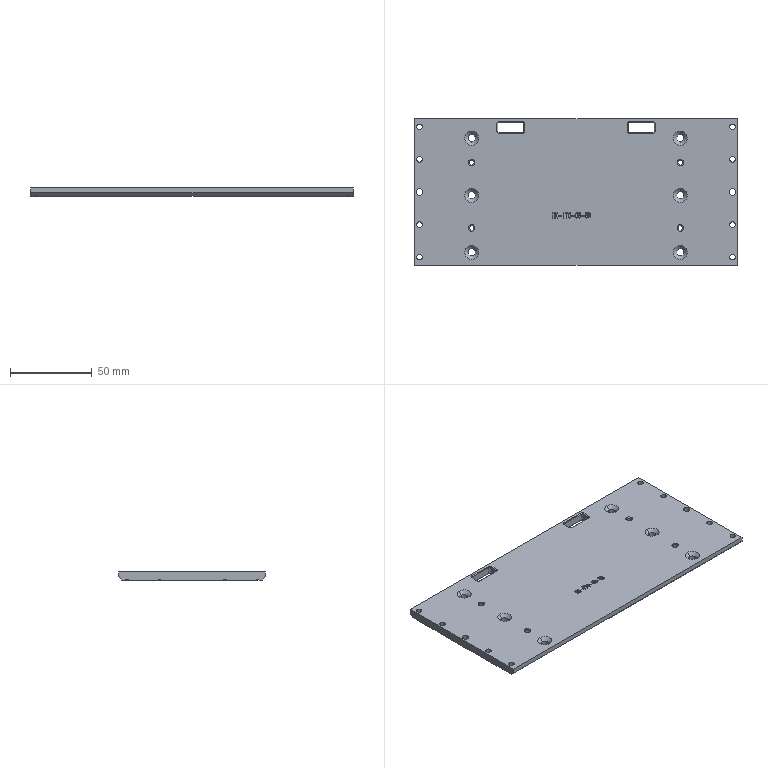NC program | NX | posted with a generic post | part box 198 x 90 x 5 mm
Lines 1 to 838 of 3871:
N10 G17 G21 G94 G90
(ZLEVEL_PROFILE_COPY_1_COPY_COPY_COPY_1_COPY , TOOL : D6A45)
N12 T01 M6
N14 G54
N16 G17 G0 G90 X65.223 Y29.3 S9500 M3
N18 G43 Z30. H1
N20 Z1.5
N22 G94 G1 X65.232 Y29.302 F1000.
N24 X65.925 Y29.611 Z1.46
N26 X66.546 Y30.049 Z1.42
N28 X67.07 Y30.598 Z1.38
N30 X67.477 Y31.239 Z1.34
N32 X67.753 Y31.946 Z1.301
N34 X67.886 Y32.694 Z1.261
N36 X67.871 Y33.453 Z1.221
N38 X67.71 Y34.195 Z1.181
N40 X67.501 Y34.712 Z1.152
N42 X67.152 Y35.293 Z1.116
N44 X66.707 Y35.804 Z1.081
N46 X66.181 Y36.23 Z1.045
N48 X65.589 Y36.559 Z1.01
N50 X64.948 Y36.78 Z0.974
N52 X64.279 Y36.887 Z0.939
N54 X63.721 Z0.91
N56 X62.989 Y36.764 Z0.871
N58 X62.293 Y36.503 Z0.832
N60 X61.659 Y36.116 Z0.793
N62 X61.111 Y35.615 Z0.754
N64 X60.767 Y35.176 Z0.725
N66 X60.406 Y34.508 Z0.685
N68 X60.182 Y33.782 Z0.645
N70 X60.103 Y33.027 Z0.605
N72 X60.172 Y32.271 Z0.566
N74 X60.386 Y31.543 Z0.526
N76 X60.737 Y30.869 Z0.486
N78 X61.212 Y30.277 Z0.446
N80 X61.792 Y29.788 Z0.406
N82 X62.457 Y29.421 Z0.367
N84 X63.18 Y29.19 Z0.327
N86 X63.733 Y29.112 Z0.298
N88 X64.492 Y29.134 Z0.258
N90 X65.232 Y29.302 Z0.218
N92 X65.925 Y29.611 Z0.178
N94 X66.546 Y30.049 Z0.138
N96 X67.07 Y30.598 Z0.099
N98 X67.477 Y31.239 Z0.059
N100 X67.753 Y31.946 Z0.019
N102 X67.886 Y32.694 Z-0.021
N104 X67.871 Y33.453 Z-0.06
N106 X67.71 Y34.195 Z-0.1
N108 X67.501 Y34.712 Z-0.129
N110 X67.152 Y35.293 Z-0.165
N112 X66.707 Y35.804 Z-0.201
N114 X66.181 Y36.23 Z-0.236
N116 X65.589 Y36.559 Z-0.272
N118 X64.948 Y36.78 Z-0.307
N120 X64.279 Y36.887 Z-0.343
N122 X64. Z-0.357
N124 G3 X60.113 Y33. R3.887 F1300.
N126 X64. Y36.887 R-3.887
N128 G1 X63.499 Y36.847 Z-0.365
N130 X63.008 Y36.742 Z-0.373
N132 X62.536 Y36.576 Z-0.38
N134 X62.09 Y36.35 Z-0.388
N136 X61.678 Y36.069 Z-0.396
N138 X61.307 Y35.738 Z-0.403
N140 X60.982 Y35.362 Z-0.411
N142 X60.689 Y34.915 Z-0.419
N144 X60.463 Y34.432 Z-0.427
N146 X60.362 Y34.127 Z-0.432
N148 X60.306 Y33.924 Z-0.435
N150 X60.263 Y33.662 Z-0.439
N152 X60.222 Y33.4 Z-0.444
N154 X60.215 Y33.135 Z-0.448
N156 X60.213 Y32.87 Z-0.452
N158 X60.24 Y32.608 Z-0.456
N160 X60.276 Y32.346 Z-0.46
N162 X60.337 Y32.09 Z-0.464
N164 X60.412 Y31.837 Z-0.468
N166 X60.506 Y31.591 Z-0.472
N168 X60.616 Y31.352 Z-0.476
N170 X60.741 Y31.122 Z-0.48
N172 X60.885 Y30.902 Z-0.484
N174 X61.042 Y30.692 Z-0.488
N176 X61.213 Y30.494 Z-0.492
N178 X61.398 Y30.31 Z-0.496
N180 X61.594 Y30.136 Z-0.5
N182 X61.804 Y29.982 Z-0.504
N184 X62.019 Y29.835 Z-0.508
N186 X62.249 Y29.713 Z-0.512
N188 X62.482 Y29.597 Z-0.516
N190 X62.727 Y29.51 Z-0.52
N192 X62.973 Y29.426 Z-0.524
N194 X63.227 Y29.375 Z-0.528
N196 X63.481 Y29.326 Z-0.532
N198 X63.739 Y29.311 Z-0.536
N200 X63.998 Y29.297 Z-0.54
N202 X64.255 Y29.319 Z-0.544
N204 X64.512 Y29.341 Z-0.548
N206 X64.817 Y29.403 Z-0.553
N208 X65.014 Y29.456 Z-0.556
N210 X65.254 Y29.546 Z-0.56
N212 X65.494 Y29.639 Z-0.564
N214 X65.719 Y29.76 Z-0.568
N216 X65.943 Y29.886 Z-0.572
N218 X66.15 Y30.036 Z-0.576
N220 X66.351 Y30.194 Z-0.579
N222 X66.537 Y30.369 Z-0.583
N224 X66.713 Y30.554 Z-0.587
N226 X66.873 Y30.752 Z-0.591
N228 X67.02 Y30.96 Z-0.595
N230 X67.153 Y31.176 Z-0.599
N232 X67.267 Y31.403 Z-0.603
N234 X67.367 Y31.636 Z-0.607
N236 X67.451 Y31.876 Z-0.611
N238 X67.515 Y32.12 Z-0.615
N240 X67.566 Y32.368 Z-0.619
N242 X67.594 Y32.619 Z-0.622
N244 X67.612 Y32.871 Z-0.626
N246 X67.603 Y33.123 Z-0.63
N248 X67.588 Y33.374 Z-0.634
N250 X67.542 Y33.621 Z-0.638
N252 X67.493 Y33.868 Z-0.642
N254 X67.413 Y34.106 Z-0.646
N256 X67.331 Y34.343 Z-0.649
N258 X67.119 Y34.766 Z-0.657
N260 X66.854 Y35.156 Z-0.664
N262 X66.621 Y35.426 Z-0.669
N264 X66.541 Y35.508 Z-0.671
N266 X66.363 Y35.662 Z-0.675
N268 X66.184 Y35.815 Z-0.678
N270 X65.988 Y35.944 Z-0.682
N272 X65.791 Y36.072 Z-0.686
N274 X65.58 Y36.173 Z-0.689
N276 X65.369 Y36.275 Z-0.693
N278 X64.924 Y36.419 Z-0.7
N280 X64.465 Y36.505 Z-0.707
N282 X64.233 Y36.516 Z-0.711
N284 X64. Y36.526 Z-0.714
N286 X63.753 Y36.507 Z-0.719
N288 X63.505 Y36.483 Z-0.723
N290 X63.263 Y36.429 Z-0.727
N292 X63.023 Y36.37 Z-0.731
N294 X62.791 Y36.284 Z-0.735
N296 X62.562 Y36.191 Z-0.74
N298 X62.344 Y36.075 Z-0.744
N300 X62.131 Y35.95 Z-0.748
N302 X61.932 Y35.806 Z-0.752
N304 X61.74 Y35.651 Z-0.756
N306 X61.562 Y35.482 Z-0.76
N308 X61.397 Y35.301 Z-0.765
N310 X61.243 Y35.11 Z-0.769
N312 X61.106 Y34.907 Z-0.773
N314 X60.983 Y34.696 Z-0.777
N316 X60.873 Y34.478 Z-0.781
N318 X60.784 Y34.251 Z-0.785
N320 X60.704 Y34.021 Z-0.79
N322 X60.646 Y33.77 Z-0.794
N324 X60.597 Y33.517 Z-0.798
N326 X60.579 Y33.26 Z-0.803
N328 X60.566 Y33.004 Z-0.807
N330 X60.587 Y32.748 Z-0.811
N332 X60.614 Y32.493 Z-0.816
N334 X60.67 Y32.244 Z-0.82
N336 X60.735 Y31.997 Z-0.825
N338 X60.826 Y31.759 Z-0.829
N340 X60.929 Y31.525 Z-0.833
N342 X61.051 Y31.302 Z-0.838
N344 X61.19 Y31.089 Z-0.842
N346 X61.346 Y30.889 Z-0.846
N348 X61.513 Y30.697 Z-0.85
N350 X61.698 Y30.525 Z-0.855
N352 X61.889 Y30.359 Z-0.859
N354 X62.098 Y30.217 Z-0.863
N356 X62.31 Y30.08 Z-0.868
N358 X62.538 Y29.973 Z-0.872
N360 X62.768 Y29.87 Z-0.876
N362 X62.898 Y29.825 Z-0.879
N364 X63.073 Y29.774 Z-0.882
N366 X63.25 Y29.73 Z-0.885
N368 X63.497 Y29.69 Z-0.889
N370 X63.746 Y29.663 Z-0.893
N372 X63.996 Y29.657 Z-0.898
N374 X64.246 Y29.671 Z-0.902
N376 X64.493 Y29.705 Z-0.906
N378 X64.737 Y29.753 Z-0.91
N380 X64.975 Y29.826 Z-0.915
N382 X65.21 Y29.907 Z-0.919
N384 X65.433 Y30.015 Z-0.923
N386 X65.654 Y30.128 Z-0.927
N388 X65.857 Y30.269 Z-0.931
N390 X66.057 Y30.415 Z-0.936
N392 X66.238 Y30.582 Z-0.94
N394 X66.413 Y30.756 Z-0.944
N396 X66.569 Y30.946 Z-0.948
N398 X66.714 Y31.145 Z-0.952
N400 X66.842 Y31.355 Z-0.957
N402 X66.952 Y31.574 Z-0.961
N404 X67.045 Y31.801 Z-0.965
N406 X67.124 Y32.033 Z-0.969
N408 X67.179 Y32.27 Z-0.973
N410 X67.225 Y32.51 Z-0.977
N412 X67.243 Y32.753 Z-0.982
N414 X67.255 Y32.996 Z-0.986
N416 X67.235 Y33.238 Z-0.99
N418 X67.21 Y33.48 Z-0.994
N420 X67.185 Y33.612 Z-0.996
N422 X67.142 Y33.782 Z-0.999
N424 X67.094 Y33.951 Z-1.002
N426 X67.008 Y34.176 Z-1.006
N428 X66.911 Y34.398 Z-1.01
N430 X66.795 Y34.609 Z-1.014
N432 X66.663 Y34.811 Z-1.019
N434 X66.516 Y35.002 Z-1.023
N436 X66.357 Y35.182 Z-1.027
N438 X66.198 Y35.334 Z-1.031
N440 X66.032 Y35.479 Z-1.034
N442 X65.853 Y35.606 Z-1.038
N444 X65.669 Y35.727 Z-1.042
N446 X65.475 Y35.828 Z-1.045
N448 X65.277 Y35.923 Z-1.049
N450 X65.071 Y35.996 Z-1.053
N452 X64.863 Y36.064 Z-1.057
N454 X64.65 Y36.107 Z-1.06
N456 X64.435 Y36.147 Z-1.064
N458 X64.218 Y36.159 Z-1.068
N460 X64. Y36.168 Z-1.071
N462 X63.775 Y36.15 Z-1.076
N464 X63.551 Y36.129 Z-1.08
N466 X63.331 Y36.079 Z-1.084
N468 X63.113 Y36.023 Z-1.089
N470 X62.903 Y35.945 Z-1.093
N472 X62.696 Y35.859 Z-1.097
N474 X62.499 Y35.753 Z-1.101
N476 X62.307 Y35.637 Z-1.106
N478 X62.127 Y35.506 Z-1.11
N480 X61.955 Y35.363 Z-1.114
N482 X61.788 Y35.201 Z-1.119
N484 X61.632 Y35.027 Z-1.123
N486 X61.494 Y34.84 Z-1.127
N488 X61.364 Y34.646 Z-1.132
N490 X61.334 Y34.595 Z-1.133
N492 X61.245 Y34.413 Z-1.137
N494 X61.156 Y34.232 Z-1.141
N496 X61.082 Y34.012 Z-1.145
N498 X61.011 Y33.792 Z-1.149
N500 X60.972 Y33.565 Z-1.154
N502 X60.937 Y33.337 Z-1.158
N504 X60.929 Y33.107 Z-1.163
N506 Y32.877 Z-1.167
N508 X60.954 Y32.649 Z-1.171
N510 X60.991 Y32.422 Z-1.176
N512 X61.046 Y32.2 Z-1.18
N514 X61.118 Y31.983 Z-1.184
N516 X61.209 Y31.774 Z-1.189
N518 X61.31 Y31.569 Z-1.193
N520 X61.432 Y31.377 Z-1.198
N522 X61.56 Y31.189 Z-1.202
N524 X61.71 Y31.019 Z-1.206
N526 X61.862 Y30.851 Z-1.21
N528 X62.036 Y30.706 Z-1.215
N530 X62.212 Y30.564 Z-1.219
N532 X62.404 Y30.445 Z-1.223
N534 X62.599 Y30.333 Z-1.228
N536 X62.805 Y30.242 Z-1.232
N538 X63.015 Y30.162 Z-1.236
N540 X63.231 Y30.1 Z-1.241
N542 X63.451 Y30.055 Z-1.245
N544 X63.673 Y30.029 Z-1.249
N546 X63.896 Y30.014 Z-1.253
N548 X63.953 Z-1.254
N550 X64.147 Y30.027 Z-1.258
N552 X64.341 Y30.041 Z-1.262
N554 X64.559 Y30.084 Z-1.266
N556 X64.777 Y30.131 Z-1.27
N558 X64.985 Y30.208 Z-1.275
N560 X65.192 Y30.288 Z-1.279
N562 X65.387 Y30.393 Z-1.283
N564 X65.578 Y30.503 Z-1.287
N566 X65.756 Y30.633 Z-1.291
N568 X65.927 Y30.773 Z-1.296
N570 X66.085 Y30.926 Z-1.3
N572 X66.231 Y31.09 Z-1.304
N574 X66.361 Y31.267 Z-1.308
N576 X66.484 Y31.448 Z-1.312
N578 X66.584 Y31.643 Z-1.316
N580 X66.68 Y31.839 Z-1.321
N582 X66.749 Y32.046 Z-1.325
N584 X66.816 Y32.254 Z-1.329
N586 X66.852 Y32.468 Z-1.333
N588 X66.887 Y32.683 Z-1.337
N590 X66.893 Y32.899 Z-1.341
N592 Y33.116 Z-1.345
N594 X66.869 Y33.331 Z-1.35
N596 X66.836 Y33.545 Z-1.354
N598 X66.78 Y33.758 Z-1.358
N600 X66.711 Y33.969 Z-1.362
N602 X66.621 Y34.17 Z-1.366
N604 X66.524 Y34.368 Z-1.371
N606 X66.508 Y34.397
N608 X66.393 Y34.565 Z-1.375
N610 X66.279 Y34.733 Z-1.379
N612 X66.132 Y34.895 Z-1.383
N614 X65.981 Y35.055 Z-1.387
N616 X65.813 Y35.193 Z-1.391
N618 X65.639 Y35.327 Z-1.396
N620 X65.453 Y35.439 Z-1.4
N622 X65.261 Y35.542 Z-1.404
N624 X65.06 Y35.626 Z-1.408
N626 X64.855 Y35.698 Z-1.412
N628 X64.644 Y35.746 Z-1.416
N630 X64.431 Y35.788 Z-1.42
N632 X64.216 Y35.803 Z-1.424
N634 X64. Y35.814 Z-1.429
N636 X63.794 Y35.795 Z-1.433
N638 X63.588 Y35.774 Z-1.438
N640 X63.387 Y35.726 Z-1.442
N642 X63.188 Y35.675 Z-1.446
N644 X62.996 Y35.6 Z-1.451
N646 X62.807 Y35.519 Z-1.455
N648 X62.629 Y35.419 Z-1.46
N650 X62.455 Y35.309 Z-1.464
N652 X62.294 Y35.184 Z-1.469
N654 X62.139 Y35.051 Z-1.473
N656 X62.014 Y34.925 Z-1.477
N658 X61.864 Y34.75 Z-1.482
N660 X61.751 Y34.581 Z-1.486
N662 X61.638 Y34.413 Z-1.491
N664 X61.537 Y34.209 Z-1.495
N666 X61.451 Y34.012 Z-1.5
N668 X61.389 Y33.801 Z-1.505
N670 X61.331 Y33.588 Z-1.51
N672 X61.3 Y33.371 Z-1.514
N674 X61.281 Y33.152 Z-1.519
N676 X61.287 Y32.933 Z-1.524
N678 X61.301 Y32.714 Z-1.529
N680 X61.344 Y32.501 Z-1.533
N682 X61.39 Y32.288 Z-1.538
N684 X61.465 Y32.078 Z-1.543
N686 X61.547 Y31.882 Z-1.547
N688 X61.652 Y31.693 Z-1.552
N690 X61.766 Y31.509 Z-1.557
N692 X61.9 Y31.339 Z-1.561
N694 X62.041 Y31.176 Z-1.566
N696 X62.201 Y31.033 Z-1.571
N698 X62.364 Y30.892 Z-1.575
N700 X62.548 Y30.771 Z-1.58
N702 X62.728 Y30.665 Z-1.585
N704 X62.924 Y30.58 Z-1.589
N706 X63.122 Y30.501 Z-1.594
N708 X63.356 Y30.435 Z-1.599
N710 X63.536 Y30.401 Z-1.603
N712 X63.747 Y30.383 Z-1.608
N714 X63.959 Y30.369 Z-1.612
N716 X64.17 Y30.386 Z-1.617
N718 X64.38 Y30.405 Z-1.621
N720 X64.59 Y30.451 Z-1.626
N722 X64.789 Y30.509 Z-1.631
N724 X64.984 Y30.587 Z-1.635
N726 X65.174 Y30.676 Z-1.64
N728 X65.352 Y30.786 Z-1.644
N730 X65.526 Y30.901 Z-1.649
N732 X65.682 Y31.04 Z-1.653
N734 X65.837 Y31.18 Z-1.658
N736 X65.974 Y31.341 Z-1.662
N738 X66.098 Y31.503 Z-1.667
N740 X66.204 Y31.681 Z-1.671
N742 X66.302 Y31.863 Z-1.676
N744 X66.378 Y32.055 Z-1.68
N746 X66.447 Y32.25 Z-1.685
N748 X66.488 Y32.451 Z-1.689
N750 X66.527 Y32.653 Z-1.693
N752 X66.539 Y32.862 Z-1.698
N754 X66.541 Y33.063 Z-1.702
N756 X66.517 Y33.266 Z-1.707
N758 X66.488 Y33.468 Z-1.711
N760 X66.431 Y33.692 Z-1.716
N762 X66.373 Y33.858 Z-1.72
N764 X66.287 Y34.042 Z-1.724
N766 X66.198 Y34.224 Z-1.729
N768 X65.981 Y34.537 Z-1.737
N770 X65.85 Y34.675 Z-1.741
N772 X65.72 Y34.813 Z-1.745
N774 X65.572 Y34.93 Z-1.749
N776 X65.421 Y35.046 Z-1.753
N778 X65.259 Y35.141 Z-1.757
N780 X65.092 Y35.229 Z-1.761
N782 X64.917 Y35.299 Z-1.766
N784 X64.74 Y35.361 Z-1.77
N786 X64.557 Y35.401 Z-1.774
N788 X64.373 Y35.438 Z-1.778
N790 X64.187 Y35.448 Z-1.782
N792 X64. Y35.459 Z-1.786
N794 X63.805 Y35.439 Z-1.791
N796 X63.609 Y35.417 Z-1.796
N798 X63.42 Y35.369 Z-1.8
N800 X63.232 Y35.314 Z-1.805
N802 X63.052 Y35.239 Z-1.81
N804 X62.877 Y35.154 Z-1.815
N806 X62.714 Y35.048 Z-1.82
N808 X62.553 Y34.94 Z-1.825
N810 X62.411 Y34.809 Z-1.83
N812 X62.269 Y34.677 Z-1.834
N814 X62.185 Y34.578 Z-1.838
N816 X62.097 Y34.463 Z-1.841
N818 X62.014 Y34.345 Z-1.845
N820 X61.912 Y34.163 Z-1.85
N822 X61.819 Y33.976 Z-1.855
N824 X61.745 Y33.765 Z-1.861
N826 X61.693 Y33.58 Z-1.866
N828 X61.662 Y33.375 Z-1.871
N830 X61.639 Y33.169 Z-1.876
N832 X61.634 Y33.02 Z-1.88
N834 X61.638 Y32.946 Z-1.882
N836 X61.654 Y32.758 Z-1.886
N838 X61.696 Y32.557 Z-1.891
N840 X61.742 Y32.357 Z-1.897
N842 X61.789 Y32.227 Z-1.9
N844 X61.836 Y32.099 Z-1.903
N846 X61.898 Y31.979 Z-1.907
N848 X62.001 Y31.804 Z-1.912
N850 X62.115 Y31.635 Z-1.917
N852 X62.257 Y31.469 Z-1.922
N854 X62.387 Y31.336 Z-1.927
N856 X62.544 Y31.209 Z-1.932
N858 X62.707 Y31.09 Z-1.937
N860 X62.829 Y31.014 Z-1.941
N862 X62.893 Y30.981 Z-1.943
N864 X62.949 Y30.955 Z-1.944
N866 X63.062 Y30.903 Z-1.947
N868 X63.252 Y30.84 Z-1.952
N870 X63.443 Y30.781 Z-1.957
N872 X63.564 Y30.758 Z-1.96
N874 X63.7 Y30.74 Z-1.964
N876 X63.837 Y30.728 Z-1.967
N878 X64.035 Y30.731 Z-1.972
N880 X64.233 Y30.744 Z-1.977
N882 X64.443 Y30.783 Z-1.982
N884 X64.618 Y30.829 Z-1.987
N886 X64.802 Y30.899 Z-1.992
N888 X64.982 Y30.978 Z-1.997
N890 X65.104 Y31.043 Z-2.
N892 X65.163 Y31.081 Z-2.002
N894 X65.213 Y31.116 Z-2.004
N896 X65.312 Y31.187 Z-2.007
N898 X65.458 Y31.316 Z-2.011
N900 X65.6 Y31.449 Z-2.016
N902 X65.688 Y31.551 Z-2.02
N904 X65.77 Y31.651 Z-2.023
N906 X65.837 Y31.756 Z-2.026
N908 X65.931 Y31.924 Z-2.031
N910 X66.016 Y32.098 Z-2.036
N912 X66.087 Y32.294 Z-2.041
N914 X66.133 Y32.464 Z-2.045
N916 X66.163 Y32.653 Z-2.05
N918 X66.184 Y32.843 Z-2.055
N920 X66.189 Y32.979 Z-2.058
N922 X66.186 Y33.046 Z-2.06
N924 X66.18 Y33.105 Z-2.061
N926 X66.169 Y33.224 Z-2.064
N928 X66.131 Y33.41 Z-2.069
N930 X66.088 Y33.594 Z-2.074
N932 X66.05 Y33.706 Z-2.077
N934 X66.004 Y33.813 Z-2.08
N936 X65.957 Y33.919 Z-2.083
N938 X65.871 Y34.071 Z-2.087
N940 X65.776 Y34.217 Z-2.091
N942 X65.667 Y34.351 Z-2.096
N944 X65.551 Y34.481 Z-2.1
N946 X65.421 Y34.594 Z-2.104
N948 X65.287 Y34.705 Z-2.109
N950 X65.141 Y34.796 Z-2.113
N952 X64.992 Y34.882 Z-2.117
N954 X64.835 Y34.95 Z-2.122
N956 X64.673 Y35.009 Z-2.126
N958 X64.508 Y35.05 Z-2.13
N960 X64.34 Y35.083 Z-2.134
N962 X64.17 Y35.095 Z-2.139
N964 X64. Y35.102 Z-2.143
N966 X63.822 Y35.085 Z-2.148
N968 X63.644 Y35.061 Z-2.153
N970 X63.521 Y35.034 Z-2.157
N972 X63.459 Y35.019 Z-2.159
N974 X63.407 Y35. Z-2.161
N976 X63.302 Y34.96 Z-2.164
N978 X63.141 Y34.886 Z-2.169
N980 X62.983 Y34.804 Z-2.174
N982 X62.826 Y34.7 Z-2.18
N984 X62.698 Y34.597 Z-2.185
N986 X62.572 Y34.474 Z-2.19
N988 X62.453 Y34.345 Z-2.195
N990 X62.345 Y34.2 Z-2.201
N992 X62.236 Y34.022 Z-2.207
N994 X62.172 Y33.891 Z-2.211
N996 X62.119 Y33.773 Z-2.215
N998 X62.085 Y33.666 Z-2.218
N1000 X62.039 Y33.479 Z-2.224
N1002 X62.005 Y33.29 Z-2.23
N1004 X61.994 Y33.152 Z-2.234
N1006 X61.989 Y33.025 Z-2.238
N1008 X61.997 Y32.908 Z-2.241
N1010 X62.023 Y32.719 Z-2.247
N1012 X62.062 Y32.533 Z-2.252
N1014 X62.103 Y32.4 Z-2.256
N1016 X62.147 Y32.282 Z-2.26
N1018 X62.195 Y32.179 Z-2.264
N1020 X62.287 Y32.015 Z-2.269
N1022 X62.392 Y31.859 Z-2.275
N1024 X62.48 Y31.75 Z-2.279
N1026 X62.565 Y31.659 Z-2.282
N1028 X62.645 Y31.583 Z-2.286
N1030 X62.79 Y31.467 Z-2.291
N1032 X62.943 Y31.361 Z-2.297
N1034 X63.061 Y31.294 Z-2.301
N1036 X63.173 Y31.243 Z-2.304
N1038 X63.277 Y31.201 Z-2.308
N1040 X63.453 Y31.149 Z-2.313
N1042 X63.632 Y31.107 Z-2.319
N1044 X63.801 Y31.087 Z-2.324
N1046 X63.997 Y31.083 Z-2.33
N1048 X64.134 Y31.092 Z-2.334
N1050 X64.255 Y31.104 Z-2.337
N1052 X64.358 Y31.127 Z-2.34
N1054 X64.532 Y31.176 Z-2.346
N1056 X64.702 Y31.238 Z-2.351
N1058 X64.823 Y31.296 Z-2.355
N1060 X64.929 Y31.353 Z-2.359
N1062 X65.017 Y31.412 Z-2.362
N1064 X65.16 Y31.519 Z-2.367
N1066 X65.292 Y31.641 Z-2.372
N1068 X65.428 Y31.794 Z-2.378
N1070 X65.517 Y31.916 Z-2.383
N1072 X65.59 Y32.031 Z-2.387
N1074 X65.623 Y32.09 Z-2.389
N1076 X65.686 Y32.227 Z-2.393
N1078 X65.758 Y32.432 Z-2.4
N1080 X65.792 Y32.562 Z-2.404
N1082 X65.824 Y32.753 Z-2.41
N1084 X65.827 Y32.805 Z-2.411
N1086 X65.832 Y32.91 Z-2.414
N1088 X65.821 Y33.136 Z-2.421
N1090 X65.808 Y33.257 Z-2.424
N1092 X65.77 Y33.426 Z-2.43
N1094 X65.715 Y33.591 Z-2.435
N1096 X65.654 Y33.738 Z-2.439
N1098 X65.579 Y33.88 Z-2.444
N1100 X65.477 Y34.025 Z-2.449
N1102 X65.391 Y34.138 Z-2.454
N1104 X65.278 Y34.256 Z-2.458
N1106 X65.163 Y34.358 Z-2.463
N1108 X65.005 Y34.468 Z-2.469
N1110 X64.902 Y34.536 Z-2.472
N1112 X64.763 Y34.599 Z-2.477
N1114 X64.614 Y34.661 Z-2.482
N1116 X64.451 Y34.706 Z-2.487
N1118 X64.31 Y34.734 Z-2.491
N1120 X64.156 Y34.749 Z-2.495
N1122 X64. Z-2.5
N1124 G3 X62.251 Y33. R1.749
N1126 X64. Y34.749 R-1.749
N1128 G1 Z-1.
N1130 G0 Z30.
N1132 X60.315 Y-3.217
N1134 Z1.5
N1136 G1 X60.386 Y-3.457 Z1.487 F1000.
N1138 X60.737 Y-4.131 Z1.447
N1140 X61.212 Y-4.723 Z1.407
N1142 X61.792 Y-5.212 Z1.367
N1144 X62.457 Y-5.579 Z1.328
N1146 X63.18 Y-5.81 Z1.288
N1148 X63.733 Y-5.888 Z1.259
N1150 X64.495 Y-5.866 Z1.219
N1152 X65.238 Y-5.696 Z1.179
N1154 X65.934 Y-5.384 Z1.139
N1156 X66.556 Y-4.943 Z1.099
N1158 X67.08 Y-4.389 Z1.059
N1160 X67.486 Y-3.743 Z1.019
N1162 X67.759 Y-3.031 Z0.979
N1164 X67.888 Y-2.279 Z0.939
N1166 Y-1.721 Z0.91
N1168 X67.826 Y-1.258 Z0.885
N1170 X67.71 Y-0.805 Z0.861
N1172 X67.501 Y-0.288 Z0.831
N1174 X67.103 Y0.358 Z0.792
N1176 X66.587 Y0.915 Z0.752
N1178 X65.973 Y1.361 Z0.712
N1180 X65.283 Y1.68 Z0.672
N1182 X64.546 Y1.859 Z0.633
N1184 X63.787 Y1.891 Z0.593
N1186 X63.037 Y1.776 Z0.553
N1188 X62.323 Y1.518 Z0.513
N1190 X61.673 Y1.126 Z0.473
N1192 X61.111 Y0.615 Z0.434
N1194 X60.767 Y0.176 Z0.404
N1196 X60.406 Y-0.492 Z0.365
N1198 X60.182 Y-1.218 Z0.325
N1200 X60.103 Y-1.973 Z0.285
N1202 X60.172 Y-2.729 Z0.245
N1204 X60.386 Y-3.457 Z0.205
N1206 X60.737 Y-4.131 Z0.166
N1208 X61.212 Y-4.723 Z0.126
N1210 X61.792 Y-5.212 Z0.086
N1212 X62.457 Y-5.579 Z0.046
N1214 X63.18 Y-5.81 Z0.006
N1216 X63.733 Y-5.888 Z-0.023
N1218 X64.495 Y-5.866 Z-0.063
N1220 X65.238 Y-5.696 Z-0.103
N1222 X65.934 Y-5.384 Z-0.143
N1224 X66.556 Y-4.943 Z-0.183
N1226 X67.08 Y-4.389 Z-0.223
N1228 X67.486 Y-3.743 Z-0.263
N1230 X67.759 Y-3.031 Z-0.303
N1232 X67.888 Y-2.279 Z-0.343
N1234 Y-2. Z-0.357
N1236 G3 X64. Y1.887 R3.887 F1300.
N1238 X67.888 Y-2. R-3.887
N1240 G1 X67.848 Y-1.506 Z-0.365
N1242 X67.747 Y-1.022 Z-0.372
N1244 X67.584 Y-0.555 Z-0.38
N1246 X67.341 Y-0.075 Z-0.388
N1248 X67.034 Y0.366 Z-0.396
N1250 X66.818 Y0.609 Z-0.401
N1252 X66.669 Y0.76 Z-0.405
N1254 X66.462 Y0.929 Z-0.409
N1256 X66.254 Y1.097 Z-0.413
N1258 X66.027 Y1.237 Z-0.417
N1260 X65.797 Y1.372 Z-0.421
N1262 X65.554 Y1.481 Z-0.425
N1264 X65.307 Y1.581 Z-0.429
N1266 X65.052 Y1.657 Z-0.433
N1268 X64.794 Y1.719 Z-0.437
N1270 X64.532 Y1.761 Z-0.442
N1272 X64.268 Y1.785 Z-0.446
N1274 X64.003 Y1.792 Z-0.45
N1276 X63.739 Y1.777 Z-0.454
N1278 X63.477 Y1.746 Z-0.458
N1280 X63.217 Y1.697 Z-0.462
N1282 X62.963 Y1.628 Z-0.466
N1284 X62.713 Y1.545 Z-0.47
N1286 X62.472 Y1.439 Z-0.474
N1288 X62.236 Y1.325 Z-0.478
N1290 X62.013 Y1.185 Z-0.482
N1292 X61.794 Y1.041 Z-0.486
N1294 X61.595 Y0.871 Z-0.49
N1296 X61.398 Y0.698 Z-0.494
N1298 X61.054 Y0.305 Z-0.502
N1300 X60.769 Y-0.131 Z-0.51
N1302 X60.548 Y-0.602 Z-0.518
N1304 X60.449 Y-0.9 Z-0.523
N1306 X60.395 Y-1.098 Z-0.526
N1308 X60.353 Y-1.354 Z-0.53
N1310 X60.313 Y-1.61 Z-0.534
N1312 X60.305 Y-1.868 Z-0.538
N1314 X60.303 Y-2.127 Z-0.542
N1316 X60.33 Y-2.383 Z-0.546
N1318 X60.365 Y-2.638 Z-0.55
N1320 X60.425 Y-2.888 Z-0.554
N1322 X60.497 Y-3.135 Z-0.558
N1324 X60.589 Y-3.375 Z-0.562
N1326 X60.697 Y-3.608 Z-0.566
N1328 X60.819 Y-3.834 Z-0.57
N1330 X60.959 Y-4.048 Z-0.574
N1332 X61.112 Y-4.253 Z-0.578
N1334 X61.279 Y-4.446 Z-0.581
N1336 X61.461 Y-4.626 Z-0.585
N1338 X61.651 Y-4.796 Z-0.589
N1340 X61.856 Y-4.946 Z-0.593
N1342 X62.067 Y-5.089 Z-0.597
N1344 X62.291 Y-5.208 Z-0.601
N1346 X62.519 Y-5.321 Z-0.605
N1348 X62.757 Y-5.407 Z-0.609
N1350 X62.997 Y-5.488 Z-0.613
N1352 X63.245 Y-5.538 Z-0.617
N1354 X63.494 Y-5.585 Z-0.62
N1356 X63.751 Y-5.601 Z-0.624
N1358 X64.008 Y-5.614 Z-0.628
N1360 X64.265 Y-5.592 Z-0.632
N1362 X64.521 Y-5.567 Z-0.636
N1364 X64.797 Y-5.511 Z-0.641
N1366 X64.909 Y-5.481 Z-0.642
N1368 X65.02 Y-5.449 Z-0.644
N1370 X65.259 Y-5.359 Z-0.648
N1372 X65.496 Y-5.262 Z-0.652
N1374 X65.721 Y-5.141 Z-0.656
N1376 X65.94 Y-5.009 Z-0.66
N1378 X66.146 Y-4.86 Z-0.664
N1380 X66.343 Y-4.697 Z-0.668
N1382 X66.527 Y-4.521 Z-0.672
N1384 X66.696 Y-4.331 Z-0.676
N1386 X66.851 Y-4.131 Z-0.679
N1388 X66.994 Y-3.921 Z-0.683
N1390 X67.116 Y-3.699 Z-0.687
N1392 X67.23 Y-3.473 Z-0.691
N1394 X67.317 Y-3.236 Z-0.695
N1396 X67.399 Y-2.997 Z-0.699
N1398 X67.451 Y-2.75 Z-0.703
N1400 X67.498 Y-2.502 Z-0.707
N1402 X67.514 Y-2.251 Z-0.71
N1404 X67.526 Y-2. Z-0.714
N1406 X67.505 Y-1.738 Z-0.719
N1408 X67.478 Y-1.477 Z-0.723
N1410 X67.451 Y-1.337 Z-0.726
N1412 X67.404 Y-1.152 Z-0.729
N1414 X67.353 Y-0.967 Z-0.732
N1416 X67.259 Y-0.723 Z-0.737
N1418 X67.153 Y-0.484 Z-0.741
N1420 X67.028 Y-0.255 Z-0.745
N1422 X66.885 Y-0.037 Z-0.75
N1424 X66.726 Y0.169 Z-0.754
N1426 X66.555 Y0.365 Z-0.759
N1428 X66.365 Y0.543 Z-0.763
N1430 X66.168 Y0.713 Z-0.768
N1432 X65.954 Y0.858 Z-0.772
N1434 X65.736 Y1. Z-0.776
N1436 X65.502 Y1.11 Z-0.781
N1438 X65.266 Y1.215 Z-0.785
N1440 X65.02 Y1.291 Z-0.79
N1442 X64.771 Y1.359 Z-0.794
N1444 X64.517 Y1.4 Z-0.798
N1446 X64.261 Y1.427 Z-0.803
N1448 X64.004 Y1.434 Z-0.807
N1450 X63.748 Y1.419 Z-0.811
N1452 X63.494 Y1.385 Z-0.816
N1454 X63.243 Y1.335 Z-0.82
N1456 X62.999 Y1.261 Z-0.825
N1458 X62.757 Y1.177 Z-0.829
N1460 X62.528 Y1.066 Z-0.833
N1462 X62.301 Y0.95 Z-0.838
N1464 X62.093 Y0.805 Z-0.842
N1466 X61.887 Y0.656 Z-0.846
N1468 X61.781 Y0.564 Z-0.849
N1470 X61.649 Y0.437 Z-0.852
N1472 X61.521 Y0.305 Z-0.855
N1474 X61.362 Y0.109 Z-0.859
N1476 X61.213 Y-0.095 Z-0.863
N1478 X61.081 Y-0.31 Z-0.868
N1480 X60.968 Y-0.536 Z-0.872
N1482 X60.873 Y-0.768 Z-0.876
N1484 X60.791 Y-1.006 Z-0.881
N1486 X60.735 Y-1.251 Z-0.885
N1488 X60.687 Y-1.497 Z-0.889
N1490 X60.669 Y-1.746 Z-0.893
N1492 X60.656 Y-1.996 Z-0.898
N1494 X60.677 Y-2.245 Z-0.902
N1496 X60.703 Y-2.493 Z-0.906
N1498 X60.758 Y-2.736 Z-0.91
N1500 X60.822 Y-2.977 Z-0.915
N1502 X60.91 Y-3.209 Z-0.919
N1504 X61.01 Y-3.436 Z-0.923
N1506 X61.129 Y-3.653 Z-0.927
N1508 X61.265 Y-3.861 Z-0.931
N1510 X61.416 Y-4.056 Z-0.936
N1512 X61.579 Y-4.242 Z-0.94
N1514 X61.759 Y-4.41 Z-0.944
N1516 X61.945 Y-4.571 Z-0.948
N1518 X62.148 Y-4.709 Z-0.952
N1520 X62.354 Y-4.843 Z-0.957
N1522 X62.576 Y-4.948 Z-0.961
N1524 X62.8 Y-5.047 Z-0.965
N1526 X62.927 Y-5.091 Z-0.967
N1528 X63.098 Y-5.14 Z-0.97
N1530 X63.27 Y-5.183 Z-0.973
N1532 X63.51 Y-5.223 Z-0.977
N1534 X63.753 Y-5.248 Z-0.982
N1536 X63.996 Y-5.255 Z-0.986
N1538 X64.239 Y-5.241 Z-0.99
N1540 X64.48 Y-5.208 Z-0.994
N1542 X64.718 Y-5.161 Z-0.998
N1544 X64.95 Y-5.091 Z-1.002
N1546 X65.178 Y-5.011 Z-1.006
N1548 X65.396 Y-4.906 Z-1.01
N1550 X65.611 Y-4.796 Z-1.015
N1552 X65.809 Y-4.658 Z-1.019
N1554 X66.004 Y-4.516 Z-1.023
N1556 X66.18 Y-4.353 Z-1.027
N1558 X66.35 Y-4.184 Z-1.031
N1560 X66.502 Y-3.998 Z-1.035
N1562 X66.643 Y-3.804 Z-1.039
N1564 X66.768 Y-3.6 Z-1.043
N1566 X66.875 Y-3.386 Z-1.047
N1568 X66.965 Y-3.165 Z-1.051
N1570 X67.042 Y-2.939 Z-1.055
N1572 X67.096 Y-2.708 Z-1.059
N1574 X67.14 Y-2.474 Z-1.063
N1576 X67.157 Y-2.237 Z-1.067
N1578 X67.168 Y-2. Z-1.071
N1580 X67.158 Y-1.85 Z-1.074
N1582 X67.148 Y-1.701 Z-1.077
N1584 X67.126 Y-1.552 Z-1.08
N1586 X67.1 Y-1.405 Z-1.083
N1588 X67.043 Y-1.176 Z-1.087
N1590 X66.968 Y-0.952 Z-1.092
N1592 X66.875 Y-0.737 Z-1.096
N1594 X66.771 Y-0.526 Z-1.101
N1596 X66.741 Y-0.474 Z-1.102
N1598 X66.628 Y-0.304 Z-1.106
N1600 X66.513 Y-0.135 Z-1.11
N1602 X66.36 Y0.042 Z-1.114
N1604 X66.203 Y0.215 Z-1.119
N1606 X66.023 Y0.364 Z-1.123
N1608 X65.841 Y0.509 Z-1.127
N1610 X65.644 Y0.632 Z-1.132
N1612 X65.443 Y0.748 Z-1.136
N1614 X65.231 Y0.842 Z-1.141
N1616 X65.014 Y0.924 Z-1.145
N1618 X64.792 Y0.988 Z-1.149
N1620 X64.565 Y1.034 Z-1.154
N1622 X64.337 Y1.061 Z-1.158
N1624 X64.107 Y1.075 Z-1.163
N1626 X63.877 Y1.066 Z-1.167
N1628 X63.648 Y1.048 Z-1.171
N1630 X63.423 Y1.004 Z-1.176
N1632 X63.199 Y0.956 Z-1.18
N1634 X62.985 Y0.876 Z-1.184
N1636 X62.772 Y0.793 Z-1.189
N1638 X62.571 Y0.686 Z-1.193
N1640 X62.374 Y0.572 Z-1.198
N1642 X62.191 Y0.438 Z-1.202
N1644 X62.015 Y0.294 Z-1.206
N1646 X61.853 Y0.136 Z-1.21
N1648 X61.701 Y-0.033 Z-1.215
N1650 X61.568 Y-0.214 Z-1.219
N1652 X61.441 Y-0.402 Z-1.223
N1654 X61.412 Y-0.452 Z-1.224
N1656 X61.239 Y-0.804 Z-1.232
N1658 X61.168 Y-1.017 Z-1.236
N1660 X61.099 Y-1.231 Z-1.241
N1662 X61.061 Y-1.452 Z-1.245
N1664 X61.026 Y-1.673 Z-1.249
N1666 X61.02 Y-1.896 Z-1.253
N1668 X61.019 Y-2.12 Z-1.258
N1670 X61.044 Y-2.341 Z-1.262
N1672 X61.078 Y-2.561 Z-1.266
N1674 X61.133 Y-2.776 Z-1.27